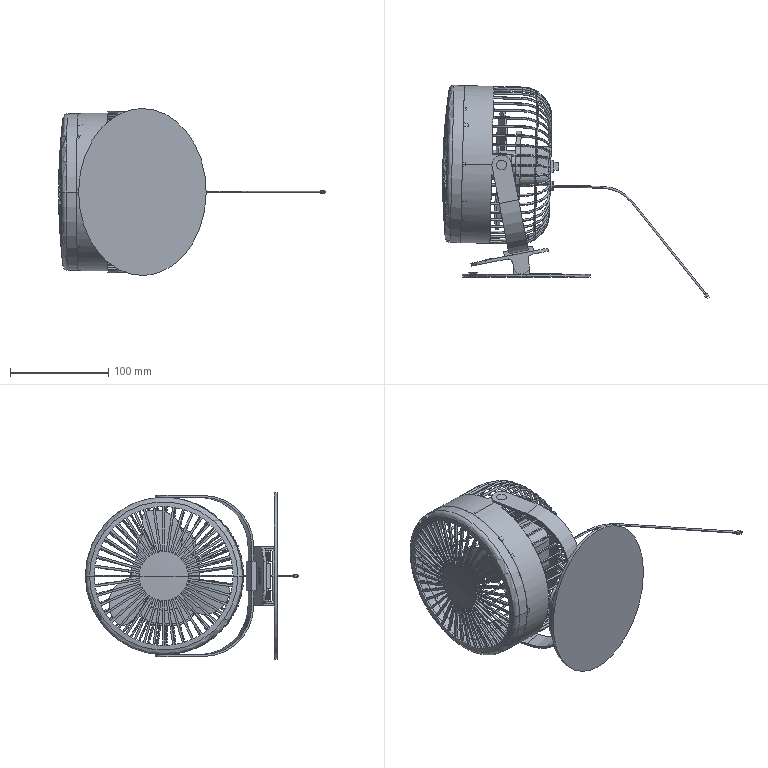Part | SolidWorks | features CompositeCurve 4 | 16 solids | 1029 faces | box 271.678 x 217.243 x 170 mm | volume 282598 mm3 | cylinder 399 | plane 388 | torus 118 | spline 76 | cone 44 | sphere 4 | commonest cylinder face diameters 2 x160 50 x44 141.176 x44 10 x30 1 x14 20 x14